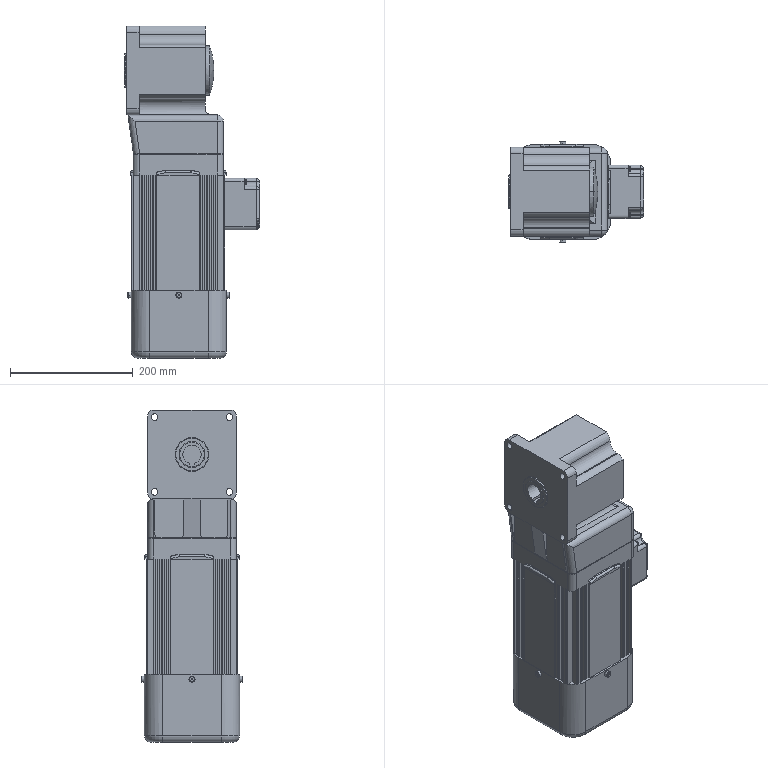Part | SolidWorks | features BaseBody 1 | 1 solid | 520 faces | box 220.628 x 166 x 541 mm | volume 11207085 mm3 | plane 361 | cylinder 105 | torus 24 | cone 22 | sphere 6 | spline 2 | commonest cylinder face diameters 20 x20 10 x16 2 x12 6 x12 9 x8 11 x8